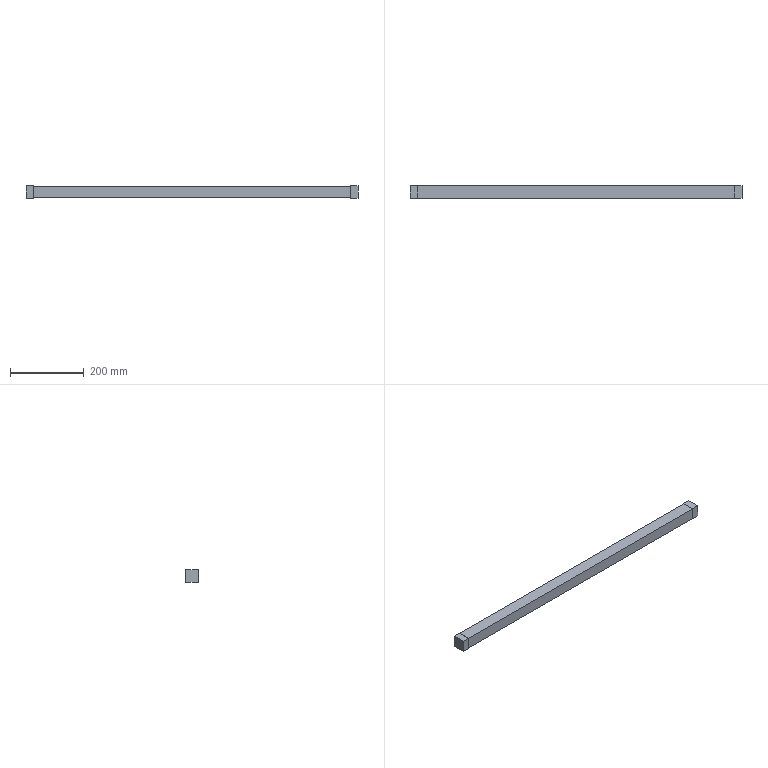Part | SolidWorks | features Extrusion 1, HoleWzd 1, ICE 1, MirrorPattern 1 | 1 solid | 24 faces | box 900 x 35 x 34 mm | volume 955428 mm3 | plane 16 | cylinder 4 | cone 4 | commonest cylinder face diameters 4.5 x4
STEP:
#1=CARTESIAN_POINT('',(-400.,6.5,-2.25));
#2=VERTEX_POINT('',#1);
#3=CARTESIAN_POINT('',(-400.,6.5,2.25));
#4=VERTEX_POINT('',#3);
#5=CARTESIAN_POINT('',(-400.,6.5,0.));
#6=DIRECTION('',(0.,1.,0.));
#7=DIRECTION('',(0.,0.,1.));
#8=AXIS2_PLACEMENT_3D('',#5,#6,#7);
#9=CIRCLE('',#8,2.25);
#10=EDGE_CURVE('',#2,#4,#9,.T.);
#11=ORIENTED_EDGE('',*,*,#10,.F.);
#12=CARTESIAN_POINT('',(-400.,16.5,-2.25));
#13=VERTEX_POINT('',#12);
#14=CARTESIAN_POINT('',(-400.,16.5,-2.25));
#15=DIRECTION('',(0.,1.,0.));
#16=VECTOR('',#15,1000.);
#17=LINE('',#14,#16);
#18=EDGE_CURVE('',#2,#13,#17,.T.);
#19=ORIENTED_EDGE('',*,*,#18,.T.);
#20=CARTESIAN_POINT('',(-400.,16.5,2.25));
#21=VERTEX_POINT('',#20);
#22=CARTESIAN_POINT('',(-400.,16.5,0.));
#23=DIRECTION('',(0.,1.,0.));
#24=DIRECTION('',(0.,0.,1.));
#25=AXIS2_PLACEMENT_3D('',#22,#23,#24);
#26=CIRCLE('',#25,2.25);
#27=EDGE_CURVE('',#13,#21,#26,.T.);
#28=ORIENTED_EDGE('',*,*,#27,.T.);
#29=CARTESIAN_POINT('',(-400.,16.5,2.25));
#30=DIRECTION('',(0.,1.,0.));
#31=VECTOR('',#30,1000.);
#32=LINE('',#29,#31);
#33=EDGE_CURVE('',#4,#21,#32,.T.);
#34=ORIENTED_EDGE('',*,*,#33,.F.);
#35=EDGE_LOOP('',(#11,#19,#28,#34));
#36=FACE_OUTER_BOUND('',#35,.T.);
#37=CARTESIAN_POINT('',(-400.,16.5,0.));
#38=DIRECTION('',(0.,1.,0.));
#39=DIRECTION('',(0.,0.,1.));
#40=AXIS2_PLACEMENT_3D('',#37,#38,#39);
#41=CYLINDRICAL_SURFACE('',#40,2.25);
#42=ADVANCED_FACE('',(#36),#41,.F.);
#43=CARTESIAN_POINT('',(-400.,5.148,0.));
#44=VERTEX_POINT('',#43);
#45=CARTESIAN_POINT('',(-400.,6.5,2.25));
#46=DIRECTION('',(0.,0.515,0.8572));
#47=VECTOR('',#46,1000.);
#48=LINE('',#45,#47);
#49=EDGE_CURVE('',#44,#4,#48,.T.);
#50=ORIENTED_EDGE('',*,*,#49,.F.);
#51=CARTESIAN_POINT('',(-400.,6.5,-2.25));
#52=DIRECTION('',(0.,0.515,-0.8572));
#53=VECTOR('',#52,1000.);
#54=LINE('',#51,#53);
#55=EDGE_CURVE('',#44,#2,#54,.T.);
#56=ORIENTED_EDGE('',*,*,#55,.T.);
#57=ORIENTED_EDGE('',*,*,#10,.T.);
#58=EDGE_LOOP('',(#50,#56,#57));
#59=FACE_OUTER_BOUND('',#58,.T.);
#60=CARTESIAN_POINT('',(-400.,6.5,0.));
#61=DIRECTION('',(0.,1.,0.));
#62=DIRECTION('',(0.,0.,1.));
#63=AXIS2_PLACEMENT_3D('',#60,#61,#62);
#64=CONICAL_SURFACE('',#63,2.25,1.03);
#65=ADVANCED_FACE('',(#59),#64,.F.);
#66=CARTESIAN_POINT('',(400.,6.5,-2.25));
#67=VERTEX_POINT('',#66);
#68=CARTESIAN_POINT('',(400.,6.5,2.25));
#69=VERTEX_POINT('',#68);
#70=CARTESIAN_POINT('',(400.,6.5,0.));
#71=DIRECTION('',(0.,1.,0.));
#72=DIRECTION('',(0.,0.,1.));
#73=AXIS2_PLACEMENT_3D('',#70,#71,#72);
#74=CIRCLE('',#73,2.25);
#75=EDGE_CURVE('',#67,#69,#74,.T.);
#76=ORIENTED_EDGE('',*,*,#75,.F.);
#77=CARTESIAN_POINT('',(400.,16.5,-2.25));
#78=VERTEX_POINT('',#77);
#79=CARTESIAN_POINT('',(400.,16.5,-2.25));
#80=DIRECTION('',(0.,1.,0.));
#81=VECTOR('',#80,1000.);
#82=LINE('',#79,#81);
#83=EDGE_CURVE('',#67,#78,#82,.T.);
#84=ORIENTED_EDGE('',*,*,#83,.T.);
#85=CARTESIAN_POINT('',(400.,16.5,2.25));
#86=VERTEX_POINT('',#85);
#87=CARTESIAN_POINT('',(400.,16.5,0.));
#88=DIRECTION('',(0.,1.,0.));
#89=DIRECTION('',(0.,0.,1.));
#90=AXIS2_PLACEMENT_3D('',#87,#88,#89);
#91=CIRCLE('',#90,2.25);
#92=EDGE_CURVE('',#78,#86,#91,.T.);
#93=ORIENTED_EDGE('',*,*,#92,.T.);
#94=CARTESIAN_POINT('',(400.,16.5,2.25));
#95=DIRECTION('',(0.,1.,0.));
#96=VECTOR('',#95,1000.);
#97=LINE('',#94,#96);
#98=EDGE_CURVE('',#69,#86,#97,.T.);
#99=ORIENTED_EDGE('',*,*,#98,.F.);
#100=EDGE_LOOP('',(#76,#84,#93,#99));
#101=FACE_OUTER_BOUND('',#100,.T.);
#102=CARTESIAN_POINT('',(400.,16.5,0.));
#103=DIRECTION('',(0.,1.,0.));
#104=DIRECTION('',(0.,0.,1.));
#105=AXIS2_PLACEMENT_3D('',#102,#103,#104);
#106=CYLINDRICAL_SURFACE('',#105,2.25);
#107=ADVANCED_FACE('',(#101),#106,.F.);
#108=CARTESIAN_POINT('',(400.,5.148,0.));
#109=VERTEX_POINT('',#108);
#110=CARTESIAN_POINT('',(400.,6.5,2.25));
#111=DIRECTION('',(0.,0.515,0.8572));
#112=VECTOR('',#111,1000.);
#113=LINE('',#110,#112);
#114=EDGE_CURVE('',#109,#69,#113,.T.);
#115=ORIENTED_EDGE('',*,*,#114,.F.);
#116=CARTESIAN_POINT('',(400.,6.5,-2.25));
#117=DIRECTION('',(0.,0.515,-0.8572));
#118=VECTOR('',#117,1000.);
#119=LINE('',#116,#118);
#120=EDGE_CURVE('',#109,#67,#119,.T.);
#121=ORIENTED_EDGE('',*,*,#120,.T.);
#122=ORIENTED_EDGE('',*,*,#75,.T.);
#123=EDGE_LOOP('',(#115,#121,#122));
#124=FACE_OUTER_BOUND('',#123,.T.);
#125=CARTESIAN_POINT('',(400.,6.5,0.));
#126=DIRECTION('',(0.,1.,0.));
#127=DIRECTION('',(0.,0.,1.));
#128=AXIS2_PLACEMENT_3D('',#125,#126,#127);
#129=CONICAL_SURFACE('',#128,2.25,1.03);
#130=ADVANCED_FACE('',(#124),#129,.F.);
#131=CARTESIAN_POINT('',(-400.,16.5,0.));
#132=DIRECTION('',(0.,1.,0.));
#133=DIRECTION('',(0.,0.,1.));
#134=AXIS2_PLACEMENT_3D('',#131,#132,#133);
#135=CIRCLE('',#134,2.25);
#136=EDGE_CURVE('',#21,#13,#135,.T.);
#137=ORIENTED_EDGE('',*,*,#136,.F.);
#138=ORIENTED_EDGE('',*,*,#27,.F.);
#139=EDGE_LOOP('',(#137,#138));
#140=FACE_BOUND('',#139,.T.);
#141=CARTESIAN_POINT('',(400.,16.5,0.));
#142=DIRECTION('',(0.,1.,0.));
#143=DIRECTION('',(0.,0.,1.));
#144=AXIS2_PLACEMENT_3D('',#141,#142,#143);
#145=CIRCLE('',#144,2.25);
#146=EDGE_CURVE('',#86,#78,#145,.T.);
#147=ORIENTED_EDGE('',*,*,#146,.F.);
#148=ORIENTED_EDGE('',*,*,#92,.F.);
#149=EDGE_LOOP('',(#147,#148));
#150=FACE_BOUND('',#149,.T.);
#151=CARTESIAN_POINT('',(-430.,16.5,16.));
#152=VERTEX_POINT('',#151);
#153=CARTESIAN_POINT('',(-430.,16.5,-16.));
#154=VERTEX_POINT('',#153);
#155=CARTESIAN_POINT('',(-430.,16.5,16.));
#156=DIRECTION('',(0.,0.,-1.));
#157=VECTOR('',#156,1000.);
#158=LINE('',#155,#157);
#159=EDGE_CURVE('',#152,#154,#158,.T.);
#160=ORIENTED_EDGE('',*,*,#159,.F.);
#161=CARTESIAN_POINT('',(430.,16.5,16.));
#162=VERTEX_POINT('',#161);
#163=CARTESIAN_POINT('',(-450.,16.5,16.));
#164=DIRECTION('',(-1.,0.,0.));
#165=VECTOR('',#164,1000.);
#166=LINE('',#163,#165);
#167=EDGE_CURVE('',#162,#152,#166,.T.);
#168=ORIENTED_EDGE('',*,*,#167,.F.);
#169=CARTESIAN_POINT('',(430.,16.5,-16.));
#170=VERTEX_POINT('',#169);
#171=CARTESIAN_POINT('',(430.,16.5,16.));
#172=DIRECTION('',(0.,0.,1.));
#173=VECTOR('',#172,1000.);
#174=LINE('',#171,#173);
#175=EDGE_CURVE('',#170,#162,#174,.T.);
#176=ORIENTED_EDGE('',*,*,#175,.F.);
#177=CARTESIAN_POINT('',(-450.,16.5,-16.));
#178=DIRECTION('',(-1.,0.,0.));
#179=VECTOR('',#178,1000.);
#180=LINE('',#177,#179);
#181=EDGE_CURVE('',#170,#154,#180,.T.);
#182=ORIENTED_EDGE('',*,*,#181,.T.);
#183=EDGE_LOOP('',(#160,#168,#176,#182));
#184=FACE_OUTER_BOUND('',#183,.T.);
#185=CARTESIAN_POINT('',(-450.,16.5,16.));
#186=DIRECTION('',(0.,-1.,0.));
#187=DIRECTION('',(0.,0.,-1.));
#188=AXIS2_PLACEMENT_3D('',#185,#186,#187);
#189=PLANE('',#188);
#190=ADVANCED_FACE('',(#140,#150,#184),#189,.F.);
#191=CARTESIAN_POINT('',(-430.,-16.5,-16.));
#192=VERTEX_POINT('',#191);
#193=CARTESIAN_POINT('',(-430.,-16.5,16.));
#194=VERTEX_POINT('',#193);
#195=CARTESIAN_POINT('',(-430.,-16.5,16.));
#196=DIRECTION('',(0.,0.,1.));
#197=VECTOR('',#196,1000.);
#198=LINE('',#195,#197);
#199=EDGE_CURVE('',#192,#194,#198,.T.);
#200=ORIENTED_EDGE('',*,*,#199,.F.);
#201=CARTESIAN_POINT('',(430.,-16.5,-16.));
#202=VERTEX_POINT('',#201);
#203=CARTESIAN_POINT('',(-450.,-16.5,-16.));
#204=DIRECTION('',(1.,0.,0.));
#205=VECTOR('',#204,1000.);
#206=LINE('',#203,#205);
#207=EDGE_CURVE('',#192,#202,#206,.T.);
#208=ORIENTED_EDGE('',*,*,#207,.T.);
#209=CARTESIAN_POINT('',(430.,-16.5,16.));
#210=VERTEX_POINT('',#209);
#211=CARTESIAN_POINT('',(430.,-16.5,16.));
#212=DIRECTION('',(0.,0.,-1.));
#213=VECTOR('',#212,1000.);
#214=LINE('',#211,#213);
#215=EDGE_CURVE('',#210,#202,#214,.T.);
#216=ORIENTED_EDGE('',*,*,#215,.F.);
#217=CARTESIAN_POINT('',(-450.,-16.5,16.));
#218=DIRECTION('',(1.,0.,0.));
#219=VECTOR('',#218,1000.);
#220=LINE('',#217,#219);
#221=EDGE_CURVE('',#194,#210,#220,.T.);
#222=ORIENTED_EDGE('',*,*,#221,.F.);
#223=EDGE_LOOP('',(#200,#208,#216,#222));
#224=FACE_OUTER_BOUND('',#223,.T.);
#225=CARTESIAN_POINT('',(-450.,-16.5,16.));
#226=DIRECTION('',(0.,1.,0.));
#227=DIRECTION('',(0.,0.,1.));
#228=AXIS2_PLACEMENT_3D('',#225,#226,#227);
#229=PLANE('',#228);
#230=ADVANCED_FACE('',(#224),#229,.F.);
#231=ORIENTED_EDGE('',*,*,#167,.T.);
#232=CARTESIAN_POINT('',(-430.,0.,16.));
#233=DIRECTION('',(0.,-1.,0.));
#234=VECTOR('',#233,1000.);
#235=LINE('',#232,#234);
#236=EDGE_CURVE('',#152,#194,#235,.T.);
#237=ORIENTED_EDGE('',*,*,#236,.T.);
#238=ORIENTED_EDGE('',*,*,#221,.T.);
#239=CARTESIAN_POINT('',(430.,0.,16.));
#240=DIRECTION('',(0.,1.,0.));
#241=VECTOR('',#240,1000.);
#242=LINE('',#239,#241);
#243=EDGE_CURVE('',#210,#162,#242,.T.);
#244=ORIENTED_EDGE('',*,*,#243,.T.);
#245=EDGE_LOOP('',(#231,#237,#238,#244));
#246=FACE_OUTER_BOUND('',#245,.T.);
#247=CARTESIAN_POINT('',(0.,0.,16.));
#248=DIRECTION('',(0.,0.,1.));
#249=DIRECTION('',(1.,0.,0.));
#250=AXIS2_PLACEMENT_3D('',#247,#248,#249);
#251=PLANE('',#250);
#252=ADVANCED_FACE('',(#246),#251,.T.);
#253=CARTESIAN_POINT('',(-430.,0.,-16.));
#254=DIRECTION('',(0.,-1.,0.));
#255=VECTOR('',#254,1000.);
#256=LINE('',#253,#255);
#257=EDGE_CURVE('',#154,#192,#256,.T.);
#258=ORIENTED_EDGE('',*,*,#257,.F.);
#259=ORIENTED_EDGE('',*,*,#181,.F.);
#260=CARTESIAN_POINT('',(430.,0.,-16.));
#261=DIRECTION('',(0.,1.,0.));
#262=VECTOR('',#261,1000.);
#263=LINE('',#260,#262);
#264=EDGE_CURVE('',#202,#170,#263,.T.);
#265=ORIENTED_EDGE('',*,*,#264,.F.);
#266=ORIENTED_EDGE('',*,*,#207,.F.);
#267=EDGE_LOOP('',(#258,#259,#265,#266));
#268=FACE_OUTER_BOUND('',#267,.T.);
#269=CARTESIAN_POINT('',(0.,0.,-16.));
#270=DIRECTION('',(0.,0.,1.));
#271=DIRECTION('',(1.,0.,0.));
#272=AXIS2_PLACEMENT_3D('',#269,#270,#271);
#273=PLANE('',#272);
#274=ADVANCED_FACE('',(#268),#273,.F.);
#275=CARTESIAN_POINT('',(450.,-17.5,-17.));
#276=VERTEX_POINT('',#275);
#277=CARTESIAN_POINT('',(450.,17.5,-17.));
#278=VERTEX_POINT('',#277);
#279=CARTESIAN_POINT('',(450.,17.5,-17.));
#280=DIRECTION('',(0.,1.,0.));
#281=VECTOR('',#280,1000.);
#282=LINE('',#279,#281);
#283=EDGE_CURVE('',#276,#278,#282,.T.);
#284=ORIENTED_EDGE('',*,*,#283,.F.);
#285=CARTESIAN_POINT('',(430.,-17.5,-17.));
#286=VERTEX_POINT('',#285);
#287=CARTESIAN_POINT('',(430.,-17.5,-17.));
#288=DIRECTION('',(1.,0.,0.));
#289=VECTOR('',#288,1000.);
#290=LINE('',#287,#289);
#291=EDGE_CURVE('',#286,#276,#290,.T.);
#292=ORIENTED_EDGE('',*,*,#291,.F.);
#293=CARTESIAN_POINT('',(430.,17.5,-17.));
#294=VERTEX_POINT('',#293);
#295=CARTESIAN_POINT('',(430.,17.5,-17.));
#296=DIRECTION('',(0.,1.,0.));
#297=VECTOR('',#296,1000.);
#298=LINE('',#295,#297);
#299=EDGE_CURVE('',#286,#294,#298,.T.);
#300=ORIENTED_EDGE('',*,*,#299,.T.);
#301=CARTESIAN_POINT('',(430.,17.5,-17.));
#302=DIRECTION('',(1.,0.,0.));
#303=VECTOR('',#302,1000.);
#304=LINE('',#301,#303);
#305=EDGE_CURVE('',#294,#278,#304,.T.);
#306=ORIENTED_EDGE('',*,*,#305,.T.);
#307=EDGE_LOOP('',(#284,#292,#300,#306));
#308=FACE_OUTER_BOUND('',#307,.T.);
#309=CARTESIAN_POINT('',(430.,17.5,-17.));
#310=DIRECTION('',(0.,0.,-1.));
#311=DIRECTION('',(-1.,0.,0.));
#312=AXIS2_PLACEMENT_3D('',#309,#310,#311);
#313=PLANE('',#312);
#314=ADVANCED_FACE('',(#308),#313,.T.);
#315=CARTESIAN_POINT('',(450.,-17.5,17.));
#316=VERTEX_POINT('',#315);
#317=CARTESIAN_POINT('',(450.,-17.5,17.));
#318=DIRECTION('',(0.,0.,-1.));
#319=VECTOR('',#318,1000.);
#320=LINE('',#317,#319);
#321=EDGE_CURVE('',#316,#276,#320,.T.);
#322=ORIENTED_EDGE('',*,*,#321,.F.);
#323=CARTESIAN_POINT('',(430.,-17.5,17.));
#324=VERTEX_POINT('',#323);
#325=CARTESIAN_POINT('',(430.,-17.5,17.));
#326=DIRECTION('',(1.,0.,0.));
#327=VECTOR('',#326,1000.);
#328=LINE('',#325,#327);
#329=EDGE_CURVE('',#324,#316,#328,.T.);
#330=ORIENTED_EDGE('',*,*,#329,.F.);
#331=CARTESIAN_POINT('',(430.,-17.5,17.));
#332=DIRECTION('',(0.,0.,-1.));
#333=VECTOR('',#332,1000.);
#334=LINE('',#331,#333);
#335=EDGE_CURVE('',#324,#286,#334,.T.);
#336=ORIENTED_EDGE('',*,*,#335,.T.);
#337=ORIENTED_EDGE('',*,*,#291,.T.);
#338=EDGE_LOOP('',(#322,#330,#336,#337));
#339=FACE_OUTER_BOUND('',#338,.T.);
#340=CARTESIAN_POINT('',(430.,-17.5,17.));
#341=DIRECTION('',(0.,-1.,0.));
#342=DIRECTION('',(0.,0.,-1.));
#343=AXIS2_PLACEMENT_3D('',#340,#341,#342);
#344=PLANE('',#343);
#345=ADVANCED_FACE('',(#339),#344,.T.);
#346=CARTESIAN_POINT('',(450.,17.5,17.));
#347=VERTEX_POINT('',#346);
#348=CARTESIAN_POINT('',(450.,17.5,17.));
#349=DIRECTION('',(0.,-1.,0.));
#350=VECTOR('',#349,1000.);
#351=LINE('',#348,#350);
#352=EDGE_CURVE('',#347,#316,#351,.T.);
#353=ORIENTED_EDGE('',*,*,#352,.F.);
#354=CARTESIAN_POINT('',(430.,17.5,17.));
#355=VERTEX_POINT('',#354);
#356=CARTESIAN_POINT('',(430.,17.5,17.));
#357=DIRECTION('',(1.,0.,0.));
#358=VECTOR('',#357,1000.);
#359=LINE('',#356,#358);
#360=EDGE_CURVE('',#355,#347,#359,.T.);
#361=ORIENTED_EDGE('',*,*,#360,.F.);
#362=CARTESIAN_POINT('',(430.,17.5,17.));
#363=DIRECTION('',(0.,-1.,0.));
#364=VECTOR('',#363,1000.);
#365=LINE('',#362,#364);
#366=EDGE_CURVE('',#355,#324,#365,.T.);
#367=ORIENTED_EDGE('',*,*,#366,.T.);
#368=ORIENTED_EDGE('',*,*,#329,.T.);
#369=EDGE_LOOP('',(#353,#361,#367,#368));
#370=FACE_OUTER_BOUND('',#369,.T.);
#371=CARTESIAN_POINT('',(430.,17.5,17.));
#372=DIRECTION('',(0.,0.,1.));
#373=DIRECTION('',(1.,0.,0.));
#374=AXIS2_PLACEMENT_3D('',#371,#372,#373);
#375=PLANE('',#374);
#376=ADVANCED_FACE('',(#370),#375,.T.);
#377=CARTESIAN_POINT('',(450.,17.5,17.));
#378=DIRECTION('',(0.,0.,1.));
#379=VECTOR('',#378,1000.);
#380=LINE('',#377,#379);
#381=EDGE_CURVE('',#278,#347,#380,.T.);
#382=ORIENTED_EDGE('',*,*,#381,.F.);
#383=ORIENTED_EDGE('',*,*,#305,.F.);
#384=CARTESIAN_POINT('',(430.,17.5,17.));
#385=DIRECTION('',(0.,0.,1.));
#386=VECTOR('',#385,1000.);
#387=LINE('',#384,#386);
#388=EDGE_CURVE('',#294,#355,#387,.T.);
#389=ORIENTED_EDGE('',*,*,#388,.T.);
#390=ORIENTED_EDGE('',*,*,#360,.T.);
#391=EDGE_LOOP('',(#382,#383,#389,#390));
#392=FACE_OUTER_BOUND('',#391,.T.);
#393=CARTESIAN_POINT('',(430.,17.5,17.));
#394=DIRECTION('',(0.,1.,0.));
#395=DIRECTION('',(0.,0.,1.));
#396=AXIS2_PLACEMENT_3D('',#393,#394,#395);
#397=PLANE('',#396);
#398=ADVANCED_FACE('',(#392),#397,.T.);
#399=ORIENTED_EDGE('',*,*,#243,.F.);
#400=ORIENTED_EDGE('',*,*,#215,.T.);
#401=ORIENTED_EDGE('',*,*,#264,.T.);
#402=ORIENTED_EDGE('',*,*,#175,.T.);
#403=EDGE_LOOP('',(#399,#400,#401,#402));
#404=FACE_BOUND('',#403,.T.);
#405=ORIENTED_EDGE('',*,*,#299,.F.);
#406=ORIENTED_EDGE('',*,*,#335,.F.);
#407=ORIENTED_EDGE('',*,*,#366,.F.);
#408=ORIENTED_EDGE('',*,*,#388,.F.);
#409=EDGE_LOOP('',(#405,#406,#407,#408));
#410=FACE_OUTER_BOUND('',#409,.T.);
#411=CARTESIAN_POINT('',(430.,0.,0.));
#412=DIRECTION('',(1.,0.,0.));
#413=DIRECTION('',(0.,0.,-1.));
#414=AXIS2_PLACEMENT_3D('',#411,#412,#413);
#415=PLANE('',#414);
#416=ADVANCED_FACE('',(#404,#410),#415,.F.);
#417=ORIENTED_EDGE('',*,*,#283,.T.);
#418=ORIENTED_EDGE('',*,*,#381,.T.);
#419=ORIENTED_EDGE('',*,*,#352,.T.);
#420=ORIENTED_EDGE('',*,*,#321,.T.);
#421=EDGE_LOOP('',(#417,#418,#419,#420));
#422=FACE_OUTER_BOUND('',#421,.T.);
#423=CARTESIAN_POINT('',(450.,16.5,16.));
#424=DIRECTION('',(-1.,0.,0.));
#425=DIRECTION('',(0.,0.,1.));
#426=AXIS2_PLACEMENT_3D('',#423,#424,#425);
#427=PLANE('',#426);
#428=ADVANCED_FACE('',(#422),#427,.F.);
#429=CARTESIAN_POINT('',(-450.,-17.5,-17.));
#430=VERTEX_POINT('',#429);
#431=CARTESIAN_POINT('',(-450.,17.5,-17.));
#432=VERTEX_POINT('',#431);
#433=CARTESIAN_POINT('',(-450.,17.5,-17.));
#434=DIRECTION('',(0.,1.,0.));
#435=VECTOR('',#434,1000.);
#436=LINE('',#433,#435);
#437=EDGE_CURVE('',#430,#432,#436,.T.);
#438=ORIENTED_EDGE('',*,*,#437,.T.);
#439=CARTESIAN_POINT('',(-430.,17.5,-17.));
#440=VERTEX_POINT('',#439);
#441=CARTESIAN_POINT('',(-430.,17.5,-17.));
#442=DIRECTION('',(-1.,0.,0.));
#443=VECTOR('',#442,1000.);
#444=LINE('',#441,#443);
#445=EDGE_CURVE('',#440,#432,#444,.T.);
#446=ORIENTED_EDGE('',*,*,#445,.F.);
#447=CARTESIAN_POINT('',(-430.,-17.5,-17.));
#448=VERTEX_POINT('',#447);
#449=CARTESIAN_POINT('',(-430.,17.5,-17.));
#450=DIRECTION('',(0.,1.,0.));
#451=VECTOR('',#450,1000.);
#452=LINE('',#449,#451);
#453=EDGE_CURVE('',#448,#440,#452,.T.);
#454=ORIENTED_EDGE('',*,*,#453,.F.);
#455=CARTESIAN_POINT('',(-430.,-17.5,-17.));
#456=DIRECTION('',(-1.,0.,0.));
#457=VECTOR('',#456,1000.);
#458=LINE('',#455,#457);
#459=EDGE_CURVE('',#448,#430,#458,.T.);
#460=ORIENTED_EDGE('',*,*,#459,.T.);
#461=EDGE_LOOP('',(#438,#446,#454,#460));
#462=FACE_OUTER_BOUND('',#461,.T.);
#463=CARTESIAN_POINT('',(-430.,17.5,-17.));
#464=DIRECTION('',(0.,0.,1.));
#465=DIRECTION('',(1.,0.,0.));
#466=AXIS2_PLACEMENT_3D('',#463,#464,#465);
#467=PLANE('',#466);
#468=ADVANCED_FACE('',(#462),#467,.F.);
#469=CARTESIAN_POINT('',(-450.,17.5,17.));
#470=VERTEX_POINT('',#469);
#471=CARTESIAN_POINT('',(-450.,17.5,17.));
#472=DIRECTION('',(0.,0.,1.));
#473=VECTOR('',#472,1000.);
#474=LINE('',#471,#473);
#475=EDGE_CURVE('',#432,#470,#474,.T.);
#476=ORIENTED_EDGE('',*,*,#475,.T.);
#477=CARTESIAN_POINT('',(-430.,17.5,17.));
#478=VERTEX_POINT('',#477);
#479=CARTESIAN_POINT('',(-430.,17.5,17.));
#480=DIRECTION('',(-1.,0.,0.));
#481=VECTOR('',#480,1000.);
#482=LINE('',#479,#481);
#483=EDGE_CURVE('',#478,#470,#482,.T.);
#484=ORIENTED_EDGE('',*,*,#483,.F.);
#485=CARTESIAN_POINT('',(-430.,17.5,17.));
#486=DIRECTION('',(0.,0.,1.));
#487=VECTOR('',#486,1000.);
#488=LINE('',#485,#487);
#489=EDGE_CURVE('',#440,#478,#488,.T.);
#490=ORIENTED_EDGE('',*,*,#489,.F.);
#491=ORIENTED_EDGE('',*,*,#445,.T.);
#492=EDGE_LOOP('',(#476,#484,#490,#491));
#493=FACE_OUTER_BOUND('',#492,.T.);
#494=CARTESIAN_POINT('',(-430.,17.5,17.));
#495=DIRECTION('',(0.,-1.,0.));
#496=DIRECTION('',(0.,0.,-1.));
#497=AXIS2_PLACEMENT_3D('',#494,#495,#496);
#498=PLANE('',#497);
#499=ADVANCED_FACE('',(#493),#498,.F.);
#500=CARTESIAN_POINT('',(-450.,-17.5,17.));
#501=VERTEX_POINT('',#500);
#502=CARTESIAN_POINT('',(-450.,17.5,17.));
#503=DIRECTION('',(0.,-1.,0.));
#504=VECTOR('',#503,1000.);
#505=LINE('',#502,#504);
#506=EDGE_CURVE('',#470,#501,#505,.T.);
#507=ORIENTED_EDGE('',*,*,#506,.T.);
#508=CARTESIAN_POINT('',(-430.,-17.5,17.));
#509=VERTEX_POINT('',#508);
#510=CARTESIAN_POINT('',(-430.,-17.5,17.));
#511=DIRECTION('',(-1.,0.,0.));
#512=VECTOR('',#511,1000.);
#513=LINE('',#510,#512);
#514=EDGE_CURVE('',#509,#501,#513,.T.);
#515=ORIENTED_EDGE('',*,*,#514,.F.);
#516=CARTESIAN_POINT('',(-430.,17.5,17.));
#517=DIRECTION('',(0.,-1.,0.));
#518=VECTOR('',#517,1000.);
#519=LINE('',#516,#518);
#520=EDGE_CURVE('',#478,#509,#519,.T.);
#521=ORIENTED_EDGE('',*,*,#520,.F.);
#522=ORIENTED_EDGE('',*,*,#483,.T.);
#523=EDGE_LOOP('',(#507,#515,#521,#522));
#524=FACE_OUTER_BOUND('',#523,.T.);
#525=CARTESIAN_POINT('',(-430.,17.5,17.));
#526=DIRECTION('',(0.,0.,-1.));
#527=DIRECTION('',(-1.,0.,0.));
#528=AXIS2_PLACEMENT_3D('',#525,#526,#527);
#529=PLANE('',#528);
#530=ADVANCED_FACE('',(#524),#529,.F.);
#531=CARTESIAN_POINT('',(-450.,-17.5,17.));
#532=DIRECTION('',(0.,0.,-1.));
#533=VECTOR('',#532,1000.);
#534=LINE('',#531,#533);
#535=EDGE_CURVE('',#501,#430,#534,.T.);
#536=ORIENTED_EDGE('',*,*,#535,.T.);
#537=ORIENTED_EDGE('',*,*,#459,.F.);
#538=CARTESIAN_POINT('',(-430.,-17.5,17.));
#539=DIRECTION('',(0.,0.,-1.));
#540=VECTOR('',#539,1000.);
#541=LINE('',#538,#540);
#542=EDGE_CURVE('',#509,#448,#541,.T.);
#543=ORIENTED_EDGE('',*,*,#542,.F.);
#544=ORIENTED_EDGE('',*,*,#514,.T.);
#545=EDGE_LOOP('',(#536,#537,#543,#544));
#546=FACE_OUTER_BOUND('',#545,.T.);
#547=CARTESIAN_POINT('',(-430.,-17.5,17.));
#548=DIRECTION('',(0.,1.,0.));
#549=DIRECTION('',(0.,0.,1.));
#550=AXIS2_PLACEMENT_3D('',#547,#548,#549);
#551=PLANE('',#550);
#552=ADVANCED_FACE('',(#546),#551,.F.);
#553=ORIENTED_EDGE('',*,*,#236,.F.);
#554=ORIENTED_EDGE('',*,*,#159,.T.);
#555=ORIENTED_EDGE('',*,*,#257,.T.);
#556=ORIENTED_EDGE('',*,*,#199,.T.);
#557=EDGE_LOOP('',(#553,#554,#555,#556));
#558=FACE_BOUND('',#557,.T.);
#559=ORIENTED_EDGE('',*,*,#453,.T.);
#560=ORIENTED_EDGE('',*,*,#489,.T.);
#561=ORIENTED_EDGE('',*,*,#520,.T.);
#562=ORIENTED_EDGE('',*,*,#542,.T.);
#563=EDGE_LOOP('',(#559,#560,#561,#562));
#564=FACE_OUTER_BOUND('',#563,.T.);
#565=CARTESIAN_POINT('',(-430.,0.,0.));
#566=DIRECTION('',(-1.,0.,0.));
#567=DIRECTION('',(0.,0.,-1.));
#568=AXIS2_PLACEMENT_3D('',#565,#566,#567);
#569=PLANE('',#568);
#570=ADVANCED_FACE('',(#558,#564),#569,.F.);
#571=ORIENTED_EDGE('',*,*,#437,.F.);
#572=ORIENTED_EDGE('',*,*,#535,.F.);
#573=ORIENTED_EDGE('',*,*,#506,.F.);
#574=ORIENTED_EDGE('',*,*,#475,.F.);
#575=EDGE_LOOP('',(#571,#572,#573,#574));
#576=FACE_OUTER_BOUND('',#575,.T.);
#577=CARTESIAN_POINT('',(-450.,16.5,16.));
#578=DIRECTION('',(1.,0.,0.));
#579=DIRECTION('',(0.,0.,-1.));
#580=AXIS2_PLACEMENT_3D('',#577,#578,#579);
#581=PLANE('',#580);
#582=ADVANCED_FACE('',(#576),#581,.F.);
#583=ORIENTED_EDGE('',*,*,#120,.F.);
#584=ORIENTED_EDGE('',*,*,#114,.T.);
#585=CARTESIAN_POINT('',(400.,6.5,0.));
#586=DIRECTION('',(0.,1.,0.));
#587=DIRECTION('',(0.,0.,1.));
#588=AXIS2_PLACEMENT_3D('',#585,#586,#587);
#589=CIRCLE('',#588,2.25);
#590=EDGE_CURVE('',#69,#67,#589,.T.);
#591=ORIENTED_EDGE('',*,*,#590,.T.);
#592=EDGE_LOOP('',(#583,#584,#591));
#593=FACE_OUTER_BOUND('',#592,.T.);
#594=CARTESIAN_POINT('',(400.,6.5,0.));
#595=DIRECTION('',(0.,1.,0.));
#596=DIRECTION('',(0.,0.,1.));
#597=AXIS2_PLACEMENT_3D('',#594,#595,#596);
#598=CONICAL_SURFACE('',#597,2.25,1.03);
#599=ADVANCED_FACE('',(#593),#598,.F.);
#600=ORIENTED_EDGE('',*,*,#83,.F.);
#601=ORIENTED_EDGE('',*,*,#590,.F.);
#602=ORIENTED_EDGE('',*,*,#98,.T.);
#603=ORIENTED_EDGE('',*,*,#146,.T.);
#604=EDGE_LOOP('',(#600,#601,#602,#603));
#605=FACE_OUTER_BOUND('',#604,.T.);
#606=CARTESIAN_POINT('',(400.,16.5,0.));
#607=DIRECTION('',(0.,1.,0.));
#608=DIRECTION('',(0.,0.,1.));
#609=AXIS2_PLACEMENT_3D('',#606,#607,#608);
#610=CYLINDRICAL_SURFACE('',#609,2.25);
#611=ADVANCED_FACE('',(#605),#610,.F.);
#612=ORIENTED_EDGE('',*,*,#55,.F.);
#613=ORIENTED_EDGE('',*,*,#49,.T.);
#614=CARTESIAN_POINT('',(-400.,6.5,0.));
#615=DIRECTION('',(0.,1.,0.));
#616=DIRECTION('',(0.,0.,1.));
#617=AXIS2_PLACEMENT_3D('',#614,#615,#616);
#618=CIRCLE('',#617,2.25);
#619=EDGE_CURVE('',#4,#2,#618,.T.);
#620=ORIENTED_EDGE('',*,*,#619,.T.);
#621=EDGE_LOOP('',(#612,#613,#620));
#622=FACE_OUTER_BOUND('',#621,.T.);
#623=CARTESIAN_POINT('',(-400.,6.5,0.));
#624=DIRECTION('',(0.,1.,0.));
#625=DIRECTION('',(0.,0.,1.));
#626=AXIS2_PLACEMENT_3D('',#623,#624,#625);
#627=CONICAL_SURFACE('',#626,2.25,1.03);
#628=ADVANCED_FACE('',(#622),#627,.F.);
#629=ORIENTED_EDGE('',*,*,#18,.F.);
#630=ORIENTED_EDGE('',*,*,#619,.F.);
#631=ORIENTED_EDGE('',*,*,#33,.T.);
#632=ORIENTED_EDGE('',*,*,#136,.T.);
#633=EDGE_LOOP('',(#629,#630,#631,#632));
#634=FACE_OUTER_BOUND('',#633,.T.);
#635=CARTESIAN_POINT('',(-400.,16.5,0.));
#636=DIRECTION('',(0.,1.,0.));
#637=DIRECTION('',(0.,0.,1.));
#638=AXIS2_PLACEMENT_3D('',#635,#636,#637);
#639=CYLINDRICAL_SURFACE('',#638,2.25);
#640=ADVANCED_FACE('',(#634),#639,.F.);
#641=CLOSED_SHELL('',(#42,#65,#107,#130,#190,#230,#252,#274,#314,#345,#376,#398,#416,#428,#468,#499,#530,#552,#570,#582,#599,#611,#628,#640));
#642=MANIFOLD_SOLID_BREP('',#641);
#643=CARTESIAN_POINT('',(0.,0.,0.));
#644=DIRECTION('',(0.,0.,1.));
#645=DIRECTION('',(1.,0.,0.));
#646=AXIS2_PLACEMENT_3D('',#643,#644,#645);
#647=(LENGTH_UNIT()NAMED_UNIT(*)SI_UNIT(.MILLI.,.METRE.));
#648=UNCERTAINTY_MEASURE_WITH_UNIT(LENGTH_MEASURE(0.00001),#647,'','');
#649=(NAMED_UNIT(*)PLANE_ANGLE_UNIT()SI_UNIT($,.RADIAN.));
#650=(NAMED_UNIT(*)SI_UNIT($,.STERADIAN.)SOLID_ANGLE_UNIT());
#651=(GEOMETRIC_REPRESENTATION_CONTEXT(3)GLOBAL_UNCERTAINTY_ASSIGNED_CONTEXT((#648))GLOBAL_UNIT_ASSIGNED_CONTEXT((#647,#649,#650))REPRESENTATION_CONTEXT('',''));
#652=ADVANCED_BREP_SHAPE_REPRESENTATION('',(#642,#646),#651);